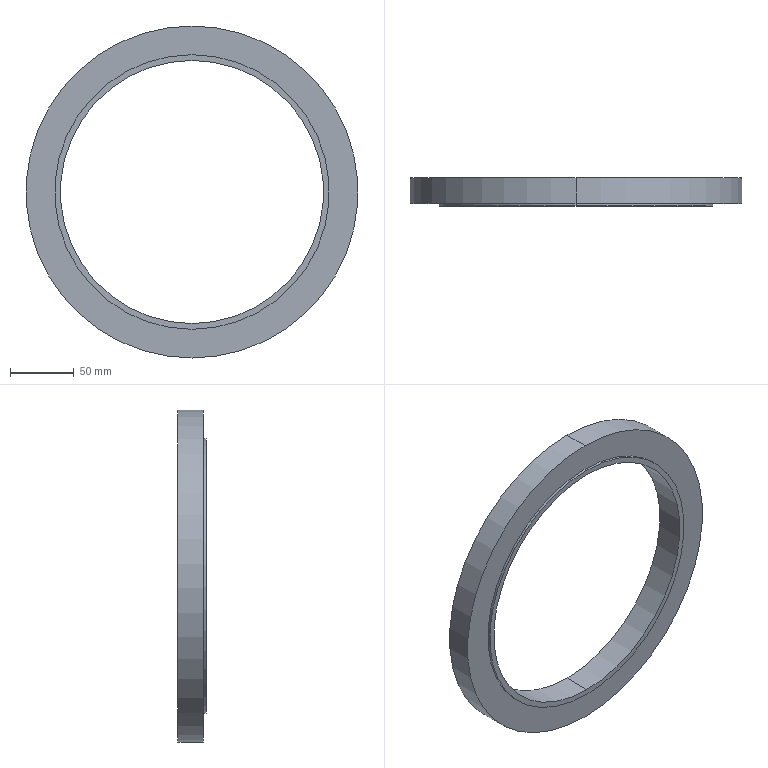Part | SolidWorks | features CirPattern 1, FlatPattern 1, HoleWzd 1, ICE 1, SMBaseFlange 1, SheetMetal 1 | 1 solid | 33 faces | box 260 x 22 x 260 mm | volume 392882 mm3 | cylinder 18 | cone 12 | plane 3 | commonest cylinder face diameters 10.2 x12 206 x2 215 x2 260 x2
STEP:
#1=CARTESIAN_POINT('',(99.593,-16.,-62.6));
#2=VERTEX_POINT('',#1);
#3=CARTESIAN_POINT('',(99.593,-16.,-52.4));
#4=VERTEX_POINT('',#3);
#5=CARTESIAN_POINT('',(99.593,-16.,-57.5));
#6=DIRECTION('',(0.,1.,0.));
#7=DIRECTION('',(0.,0.,1.));
#8=AXIS2_PLACEMENT_3D('',#5,#6,#7);
#9=CIRCLE('',#8,5.1);
#10=EDGE_CURVE('',#2,#4,#9,.T.);
#11=ORIENTED_EDGE('',*,*,#10,.F.);
#12=CARTESIAN_POINT('',(99.593,0.,-62.6));
#13=VERTEX_POINT('',#12);
#14=CARTESIAN_POINT('',(99.593,0.,-62.6));
#15=DIRECTION('',(0.,1.,0.));
#16=VECTOR('',#15,1000.);
#17=LINE('',#14,#16);
#18=EDGE_CURVE('',#2,#13,#17,.T.);
#19=ORIENTED_EDGE('',*,*,#18,.T.);
#20=CARTESIAN_POINT('',(99.593,0.,-52.4));
#21=VERTEX_POINT('',#20);
#22=CARTESIAN_POINT('',(99.593,0.,-57.5));
#23=DIRECTION('',(0.,1.,0.));
#24=DIRECTION('',(0.,0.,1.));
#25=AXIS2_PLACEMENT_3D('',#22,#23,#24);
#26=CIRCLE('',#25,5.1);
#27=EDGE_CURVE('',#13,#21,#26,.T.);
#28=ORIENTED_EDGE('',*,*,#27,.T.);
#29=CARTESIAN_POINT('',(99.593,0.,-52.4));
#30=DIRECTION('',(0.,1.,0.));
#31=VECTOR('',#30,1000.);
#32=LINE('',#29,#31);
#33=EDGE_CURVE('',#4,#21,#32,.T.);
#34=ORIENTED_EDGE('',*,*,#33,.F.);
#35=EDGE_LOOP('',(#11,#19,#28,#34));
#36=FACE_OUTER_BOUND('',#35,.T.);
#37=CARTESIAN_POINT('',(99.593,0.,-57.5));
#38=DIRECTION('',(0.,1.,0.));
#39=DIRECTION('',(0.,0.,1.));
#40=AXIS2_PLACEMENT_3D('',#37,#38,#39);
#41=CYLINDRICAL_SURFACE('',#40,5.1);
#42=ADVANCED_FACE('',(#36),#41,.F.);
#43=CARTESIAN_POINT('',(99.593,-19.064,-57.5));
#44=VERTEX_POINT('',#43);
#45=CARTESIAN_POINT('',(99.593,-16.,-52.4));
#46=DIRECTION('',(0.,0.515,0.8572));
#47=VECTOR('',#46,1000.);
#48=LINE('',#45,#47);
#49=EDGE_CURVE('',#44,#4,#48,.T.);
#50=ORIENTED_EDGE('',*,*,#49,.F.);
#51=CARTESIAN_POINT('',(99.593,-16.,-62.6));
#52=DIRECTION('',(0.,0.515,-0.8572));
#53=VECTOR('',#52,1000.);
#54=LINE('',#51,#53);
#55=EDGE_CURVE('',#44,#2,#54,.T.);
#56=ORIENTED_EDGE('',*,*,#55,.T.);
#57=ORIENTED_EDGE('',*,*,#10,.T.);
#58=EDGE_LOOP('',(#50,#56,#57));
#59=FACE_OUTER_BOUND('',#58,.T.);
#60=CARTESIAN_POINT('',(99.593,-16.,-57.5));
#61=DIRECTION('',(0.,1.,0.));
#62=DIRECTION('',(0.,0.,1.));
#63=AXIS2_PLACEMENT_3D('',#60,#61,#62);
#64=CONICAL_SURFACE('',#63,5.1,1.03);
#65=ADVANCED_FACE('',(#59),#64,.F.);
#66=CARTESIAN_POINT('',(99.593,-16.,52.4));
#67=VERTEX_POINT('',#66);
#68=CARTESIAN_POINT('',(99.593,-16.,62.6));
#69=VERTEX_POINT('',#68);
#70=CARTESIAN_POINT('',(99.593,-16.,57.5));
#71=DIRECTION('',(0.,1.,0.));
#72=DIRECTION('',(0.,0.,1.));
#73=AXIS2_PLACEMENT_3D('',#70,#71,#72);
#74=CIRCLE('',#73,5.1);
#75=EDGE_CURVE('',#67,#69,#74,.T.);
#76=ORIENTED_EDGE('',*,*,#75,.F.);
#77=CARTESIAN_POINT('',(99.593,0.,52.4));
#78=VERTEX_POINT('',#77);
#79=CARTESIAN_POINT('',(99.593,0.,52.4));
#80=DIRECTION('',(0.,1.,0.));
#81=VECTOR('',#80,1000.);
#82=LINE('',#79,#81);
#83=EDGE_CURVE('',#67,#78,#82,.T.);
#84=ORIENTED_EDGE('',*,*,#83,.T.);
#85=CARTESIAN_POINT('',(99.593,0.,62.6));
#86=VERTEX_POINT('',#85);
#87=CARTESIAN_POINT('',(99.593,0.,57.5));
#88=DIRECTION('',(0.,1.,0.));
#89=DIRECTION('',(0.,0.,1.));
#90=AXIS2_PLACEMENT_3D('',#87,#88,#89);
#91=CIRCLE('',#90,5.1);
#92=EDGE_CURVE('',#78,#86,#91,.T.);
#93=ORIENTED_EDGE('',*,*,#92,.T.);
#94=CARTESIAN_POINT('',(99.593,0.,62.6));
#95=DIRECTION('',(0.,1.,0.));
#96=VECTOR('',#95,1000.);
#97=LINE('',#94,#96);
#98=EDGE_CURVE('',#69,#86,#97,.T.);
#99=ORIENTED_EDGE('',*,*,#98,.F.);
#100=EDGE_LOOP('',(#76,#84,#93,#99));
#101=FACE_OUTER_BOUND('',#100,.T.);
#102=CARTESIAN_POINT('',(99.593,0.,57.5));
#103=DIRECTION('',(0.,1.,0.));
#104=DIRECTION('',(0.,0.,1.));
#105=AXIS2_PLACEMENT_3D('',#102,#103,#104);
#106=CYLINDRICAL_SURFACE('',#105,5.1);
#107=ADVANCED_FACE('',(#101),#106,.F.);
#108=CARTESIAN_POINT('',(99.593,-19.064,57.5));
#109=VERTEX_POINT('',#108);
#110=CARTESIAN_POINT('',(99.593,-16.,62.6));
#111=DIRECTION('',(0.,0.515,0.8572));
#112=VECTOR('',#111,1000.);
#113=LINE('',#110,#112);
#114=EDGE_CURVE('',#109,#69,#113,.T.);
#115=ORIENTED_EDGE('',*,*,#114,.F.);
#116=CARTESIAN_POINT('',(99.593,-16.,52.4));
#117=DIRECTION('',(0.,0.515,-0.8572));
#118=VECTOR('',#117,1000.);
#119=LINE('',#116,#118);
#120=EDGE_CURVE('',#109,#67,#119,.T.);
#121=ORIENTED_EDGE('',*,*,#120,.T.);
#122=ORIENTED_EDGE('',*,*,#75,.T.);
#123=EDGE_LOOP('',(#115,#121,#122));
#124=FACE_OUTER_BOUND('',#123,.T.);
#125=CARTESIAN_POINT('',(99.593,-16.,57.5));
#126=DIRECTION('',(0.,1.,0.));
#127=DIRECTION('',(0.,0.,1.));
#128=AXIS2_PLACEMENT_3D('',#125,#126,#127);
#129=CONICAL_SURFACE('',#128,5.1,1.03);
#130=ADVANCED_FACE('',(#124),#129,.F.);
#131=CARTESIAN_POINT('',(0.,-16.,109.9));
#132=VERTEX_POINT('',#131);
#133=CARTESIAN_POINT('',(0.,-16.,120.1));
#134=VERTEX_POINT('',#133);
#135=CARTESIAN_POINT('',(0.,-16.,115.));
#136=DIRECTION('',(0.,1.,0.));
#137=DIRECTION('',(0.,0.,1.));
#138=AXIS2_PLACEMENT_3D('',#135,#136,#137);
#139=CIRCLE('',#138,5.1);
#140=EDGE_CURVE('',#132,#134,#139,.T.);
#141=ORIENTED_EDGE('',*,*,#140,.F.);
#142=CARTESIAN_POINT('',(0.,0.,109.9));
#143=VERTEX_POINT('',#142);
#144=CARTESIAN_POINT('',(0.,0.,109.9));
#145=DIRECTION('',(0.,1.,0.));
#146=VECTOR('',#145,1000.);
#147=LINE('',#144,#146);
#148=EDGE_CURVE('',#132,#143,#147,.T.);
#149=ORIENTED_EDGE('',*,*,#148,.T.);
#150=CARTESIAN_POINT('',(0.,0.,120.1));
#151=VERTEX_POINT('',#150);
#152=CARTESIAN_POINT('',(0.,0.,115.));
#153=DIRECTION('',(0.,1.,0.));
#154=DIRECTION('',(0.,0.,1.));
#155=AXIS2_PLACEMENT_3D('',#152,#153,#154);
#156=CIRCLE('',#155,5.1);
#157=EDGE_CURVE('',#143,#151,#156,.T.);
#158=ORIENTED_EDGE('',*,*,#157,.T.);
#159=CARTESIAN_POINT('',(0.,0.,120.1));
#160=DIRECTION('',(0.,1.,0.));
#161=VECTOR('',#160,1000.);
#162=LINE('',#159,#161);
#163=EDGE_CURVE('',#134,#151,#162,.T.);
#164=ORIENTED_EDGE('',*,*,#163,.F.);
#165=EDGE_LOOP('',(#141,#149,#158,#164));
#166=FACE_OUTER_BOUND('',#165,.T.);
#167=CARTESIAN_POINT('',(0.,0.,115.));
#168=DIRECTION('',(0.,1.,0.));
#169=DIRECTION('',(0.,0.,1.));
#170=AXIS2_PLACEMENT_3D('',#167,#168,#169);
#171=CYLINDRICAL_SURFACE('',#170,5.1);
#172=ADVANCED_FACE('',(#166),#171,.F.);
#173=CARTESIAN_POINT('',(0.,-19.064,115.));
#174=VERTEX_POINT('',#173);
#175=CARTESIAN_POINT('',(0.,-16.,120.1));
#176=DIRECTION('',(0.,0.515,0.8572));
#177=VECTOR('',#176,1000.);
#178=LINE('',#175,#177);
#179=EDGE_CURVE('',#174,#134,#178,.T.);
#180=ORIENTED_EDGE('',*,*,#179,.F.);
#181=CARTESIAN_POINT('',(0.,-16.,109.9));
#182=DIRECTION('',(0.,0.515,-0.8572));
#183=VECTOR('',#182,1000.);
#184=LINE('',#181,#183);
#185=EDGE_CURVE('',#174,#132,#184,.T.);
#186=ORIENTED_EDGE('',*,*,#185,.T.);
#187=ORIENTED_EDGE('',*,*,#140,.T.);
#188=EDGE_LOOP('',(#180,#186,#187));
#189=FACE_OUTER_BOUND('',#188,.T.);
#190=CARTESIAN_POINT('',(0.,-16.,115.));
#191=DIRECTION('',(0.,1.,0.));
#192=DIRECTION('',(0.,0.,1.));
#193=AXIS2_PLACEMENT_3D('',#190,#191,#192);
#194=CONICAL_SURFACE('',#193,5.1,1.03);
#195=ADVANCED_FACE('',(#189),#194,.F.);
#196=CARTESIAN_POINT('',(-99.593,-16.,52.4));
#197=VERTEX_POINT('',#196);
#198=CARTESIAN_POINT('',(-99.593,-16.,62.6));
#199=VERTEX_POINT('',#198);
#200=CARTESIAN_POINT('',(-99.593,-16.,57.5));
#201=DIRECTION('',(0.,1.,0.));
#202=DIRECTION('',(0.,0.,1.));
#203=AXIS2_PLACEMENT_3D('',#200,#201,#202);
#204=CIRCLE('',#203,5.1);
#205=EDGE_CURVE('',#197,#199,#204,.T.);
#206=ORIENTED_EDGE('',*,*,#205,.F.);
#207=CARTESIAN_POINT('',(-99.593,0.,52.4));
#208=VERTEX_POINT('',#207);
#209=CARTESIAN_POINT('',(-99.593,0.,52.4));
#210=DIRECTION('',(0.,1.,0.));
#211=VECTOR('',#210,1000.);
#212=LINE('',#209,#211);
#213=EDGE_CURVE('',#197,#208,#212,.T.);
#214=ORIENTED_EDGE('',*,*,#213,.T.);
#215=CARTESIAN_POINT('',(-99.593,0.,62.6));
#216=VERTEX_POINT('',#215);
#217=CARTESIAN_POINT('',(-99.593,0.,57.5));
#218=DIRECTION('',(0.,1.,0.));
#219=DIRECTION('',(0.,0.,1.));
#220=AXIS2_PLACEMENT_3D('',#217,#218,#219);
#221=CIRCLE('',#220,5.1);
#222=EDGE_CURVE('',#208,#216,#221,.T.);
#223=ORIENTED_EDGE('',*,*,#222,.T.);
#224=CARTESIAN_POINT('',(-99.593,0.,62.6));
#225=DIRECTION('',(0.,1.,0.));
#226=VECTOR('',#225,1000.);
#227=LINE('',#224,#226);
#228=EDGE_CURVE('',#199,#216,#227,.T.);
#229=ORIENTED_EDGE('',*,*,#228,.F.);
#230=EDGE_LOOP('',(#206,#214,#223,#229));
#231=FACE_OUTER_BOUND('',#230,.T.);
#232=CARTESIAN_POINT('',(-99.593,0.,57.5));
#233=DIRECTION('',(0.,1.,0.));
#234=DIRECTION('',(0.,0.,1.));
#235=AXIS2_PLACEMENT_3D('',#232,#233,#234);
#236=CYLINDRICAL_SURFACE('',#235,5.1);
#237=ADVANCED_FACE('',(#231),#236,.F.);
#238=CARTESIAN_POINT('',(-99.593,-19.064,57.5));
#239=VERTEX_POINT('',#238);
#240=CARTESIAN_POINT('',(-99.593,-16.,62.6));
#241=DIRECTION('',(0.,0.515,0.8572));
#242=VECTOR('',#241,1000.);
#243=LINE('',#240,#242);
#244=EDGE_CURVE('',#239,#199,#243,.T.);
#245=ORIENTED_EDGE('',*,*,#244,.F.);
#246=CARTESIAN_POINT('',(-99.593,-16.,52.4));
#247=DIRECTION('',(0.,0.515,-0.8572));
#248=VECTOR('',#247,1000.);
#249=LINE('',#246,#248);
#250=EDGE_CURVE('',#239,#197,#249,.T.);
#251=ORIENTED_EDGE('',*,*,#250,.T.);
#252=ORIENTED_EDGE('',*,*,#205,.T.);
#253=EDGE_LOOP('',(#245,#251,#252));
#254=FACE_OUTER_BOUND('',#253,.T.);
#255=CARTESIAN_POINT('',(-99.593,-16.,57.5));
#256=DIRECTION('',(0.,1.,0.));
#257=DIRECTION('',(0.,0.,1.));
#258=AXIS2_PLACEMENT_3D('',#255,#256,#257);
#259=CONICAL_SURFACE('',#258,5.1,1.03);
#260=ADVANCED_FACE('',(#254),#259,.F.);
#261=CARTESIAN_POINT('',(-99.593,-16.,-62.6));
#262=VERTEX_POINT('',#261);
#263=CARTESIAN_POINT('',(-99.593,-16.,-52.4));
#264=VERTEX_POINT('',#263);
#265=CARTESIAN_POINT('',(-99.593,-16.,-57.5));
#266=DIRECTION('',(0.,1.,0.));
#267=DIRECTION('',(0.,0.,1.));
#268=AXIS2_PLACEMENT_3D('',#265,#266,#267);
#269=CIRCLE('',#268,5.1);
#270=EDGE_CURVE('',#262,#264,#269,.T.);
#271=ORIENTED_EDGE('',*,*,#270,.F.);
#272=CARTESIAN_POINT('',(-99.593,0.,-62.6));
#273=VERTEX_POINT('',#272);
#274=CARTESIAN_POINT('',(-99.593,0.,-62.6));
#275=DIRECTION('',(0.,1.,0.));
#276=VECTOR('',#275,1000.);
#277=LINE('',#274,#276);
#278=EDGE_CURVE('',#262,#273,#277,.T.);
#279=ORIENTED_EDGE('',*,*,#278,.T.);
#280=CARTESIAN_POINT('',(-99.593,0.,-52.4));
#281=VERTEX_POINT('',#280);
#282=CARTESIAN_POINT('',(-99.593,0.,-57.5));
#283=DIRECTION('',(0.,1.,0.));
#284=DIRECTION('',(0.,0.,1.));
#285=AXIS2_PLACEMENT_3D('',#282,#283,#284);
#286=CIRCLE('',#285,5.1);
#287=EDGE_CURVE('',#273,#281,#286,.T.);
#288=ORIENTED_EDGE('',*,*,#287,.T.);
#289=CARTESIAN_POINT('',(-99.593,0.,-52.4));
#290=DIRECTION('',(0.,1.,0.));
#291=VECTOR('',#290,1000.);
#292=LINE('',#289,#291);
#293=EDGE_CURVE('',#264,#281,#292,.T.);
#294=ORIENTED_EDGE('',*,*,#293,.F.);
#295=EDGE_LOOP('',(#271,#279,#288,#294));
#296=FACE_OUTER_BOUND('',#295,.T.);
#297=CARTESIAN_POINT('',(-99.593,0.,-57.5));
#298=DIRECTION('',(0.,1.,0.));
#299=DIRECTION('',(0.,0.,1.));
#300=AXIS2_PLACEMENT_3D('',#297,#298,#299);
#301=CYLINDRICAL_SURFACE('',#300,5.1);
#302=ADVANCED_FACE('',(#296),#301,.F.);
#303=CARTESIAN_POINT('',(-99.593,-19.064,-57.5));
#304=VERTEX_POINT('',#303);
#305=CARTESIAN_POINT('',(-99.593,-16.,-52.4));
#306=DIRECTION('',(0.,0.515,0.8572));
#307=VECTOR('',#306,1000.);
#308=LINE('',#305,#307);
#309=EDGE_CURVE('',#304,#264,#308,.T.);
#310=ORIENTED_EDGE('',*,*,#309,.F.);
#311=CARTESIAN_POINT('',(-99.593,-16.,-62.6));
#312=DIRECTION('',(0.,0.515,-0.8572));
#313=VECTOR('',#312,1000.);
#314=LINE('',#311,#313);
#315=EDGE_CURVE('',#304,#262,#314,.T.);
#316=ORIENTED_EDGE('',*,*,#315,.T.);
#317=ORIENTED_EDGE('',*,*,#270,.T.);
#318=EDGE_LOOP('',(#310,#316,#317));
#319=FACE_OUTER_BOUND('',#318,.T.);
#320=CARTESIAN_POINT('',(-99.593,-16.,-57.5));
#321=DIRECTION('',(0.,1.,0.));
#322=DIRECTION('',(0.,0.,1.));
#323=AXIS2_PLACEMENT_3D('',#320,#321,#322);
#324=CONICAL_SURFACE('',#323,5.1,1.03);
#325=ADVANCED_FACE('',(#319),#324,.F.);
#326=CARTESIAN_POINT('',(0.,-16.,-120.1));
#327=VERTEX_POINT('',#326);
#328=CARTESIAN_POINT('',(0.,-16.,-109.9));
#329=VERTEX_POINT('',#328);
#330=CARTESIAN_POINT('',(0.,-16.,-115.));
#331=DIRECTION('',(0.,1.,0.));
#332=DIRECTION('',(0.,0.,1.));
#333=AXIS2_PLACEMENT_3D('',#330,#331,#332);
#334=CIRCLE('',#333,5.1);
#335=EDGE_CURVE('',#327,#329,#334,.T.);
#336=ORIENTED_EDGE('',*,*,#335,.F.);
#337=CARTESIAN_POINT('',(0.,0.,-120.1));
#338=VERTEX_POINT('',#337);
#339=CARTESIAN_POINT('',(0.,0.,-120.1));
#340=DIRECTION('',(0.,1.,0.));
#341=VECTOR('',#340,1000.);
#342=LINE('',#339,#341);
#343=EDGE_CURVE('',#327,#338,#342,.T.);
#344=ORIENTED_EDGE('',*,*,#343,.T.);
#345=CARTESIAN_POINT('',(0.,0.,-109.9));
#346=VERTEX_POINT('',#345);
#347=CARTESIAN_POINT('',(0.,0.,-115.));
#348=DIRECTION('',(0.,1.,0.));
#349=DIRECTION('',(0.,0.,1.));
#350=AXIS2_PLACEMENT_3D('',#347,#348,#349);
#351=CIRCLE('',#350,5.1);
#352=EDGE_CURVE('',#338,#346,#351,.T.);
#353=ORIENTED_EDGE('',*,*,#352,.T.);
#354=CARTESIAN_POINT('',(0.,0.,-109.9));
#355=DIRECTION('',(0.,1.,0.));
#356=VECTOR('',#355,1000.);
#357=LINE('',#354,#356);
#358=EDGE_CURVE('',#329,#346,#357,.T.);
#359=ORIENTED_EDGE('',*,*,#358,.F.);
#360=EDGE_LOOP('',(#336,#344,#353,#359));
#361=FACE_OUTER_BOUND('',#360,.T.);
#362=CARTESIAN_POINT('',(0.,0.,-115.));
#363=DIRECTION('',(0.,1.,0.));
#364=DIRECTION('',(0.,0.,1.));
#365=AXIS2_PLACEMENT_3D('',#362,#363,#364);
#366=CYLINDRICAL_SURFACE('',#365,5.1);
#367=ADVANCED_FACE('',(#361),#366,.F.);
#368=CARTESIAN_POINT('',(0.,-19.064,-115.));
#369=VERTEX_POINT('',#368);
#370=CARTESIAN_POINT('',(0.,-16.,-109.9));
#371=DIRECTION('',(0.,0.515,0.8572));
#372=VECTOR('',#371,1000.);
#373=LINE('',#370,#372);
#374=EDGE_CURVE('',#369,#329,#373,.T.);
#375=ORIENTED_EDGE('',*,*,#374,.F.);
#376=CARTESIAN_POINT('',(0.,-16.,-120.1));
#377=DIRECTION('',(0.,0.515,-0.8572));
#378=VECTOR('',#377,1000.);
#379=LINE('',#376,#378);
#380=EDGE_CURVE('',#369,#327,#379,.T.);
#381=ORIENTED_EDGE('',*,*,#380,.T.);
#382=ORIENTED_EDGE('',*,*,#335,.T.);
#383=EDGE_LOOP('',(#375,#381,#382));
#384=FACE_OUTER_BOUND('',#383,.T.);
#385=CARTESIAN_POINT('',(0.,-16.,-115.));
#386=DIRECTION('',(0.,1.,0.));
#387=DIRECTION('',(0.,0.,1.));
#388=AXIS2_PLACEMENT_3D('',#385,#386,#387);
#389=CONICAL_SURFACE('',#388,5.1,1.03);
#390=ADVANCED_FACE('',(#384),#389,.F.);
#391=CARTESIAN_POINT('',(0.,-20.,-107.5));
#392=VERTEX_POINT('',#391);
#393=CARTESIAN_POINT('',(0.,-20.,107.5));
#394=VERTEX_POINT('',#393);
#395=CARTESIAN_POINT('',(0.,-20.,0.));
#396=DIRECTION('',(0.,-1.,0.));
#397=DIRECTION('',(0.,0.,-1.));
#398=AXIS2_PLACEMENT_3D('',#395,#396,#397);
#399=CIRCLE('',#398,107.5);
#400=EDGE_CURVE('',#392,#394,#399,.T.);
#401=ORIENTED_EDGE('',*,*,#400,.T.);
#402=CARTESIAN_POINT('',(0.,-22.,107.5));
#403=VERTEX_POINT('',#402);
#404=CARTESIAN_POINT('',(0.,-20.,107.5));
#405=DIRECTION('',(0.,-1.,0.));
#406=VECTOR('',#405,1000.);
#407=LINE('',#404,#406);
#408=EDGE_CURVE('',#394,#403,#407,.T.);
#409=ORIENTED_EDGE('',*,*,#408,.T.);
#410=CARTESIAN_POINT('',(0.,-22.,-107.5));
#411=VERTEX_POINT('',#410);
#412=CARTESIAN_POINT('',(0.,-22.,0.));
#413=DIRECTION('',(0.,-1.,0.));
#414=DIRECTION('',(0.,0.,-1.));
#415=AXIS2_PLACEMENT_3D('',#412,#413,#414);
#416=CIRCLE('',#415,107.5);
#417=EDGE_CURVE('',#411,#403,#416,.T.);
#418=ORIENTED_EDGE('',*,*,#417,.F.);
#419=CARTESIAN_POINT('',(0.,-20.,-107.5));
#420=DIRECTION('',(0.,-1.,0.));
#421=VECTOR('',#420,1000.);
#422=LINE('',#419,#421);
#423=EDGE_CURVE('',#392,#411,#422,.T.);
#424=ORIENTED_EDGE('',*,*,#423,.F.);
#425=EDGE_LOOP('',(#401,#409,#418,#424));
#426=FACE_OUTER_BOUND('',#425,.T.);
#427=CARTESIAN_POINT('',(0.,-20.,0.));
#428=DIRECTION('',(0.,-1.,0.));
#429=DIRECTION('',(0.,0.,-1.));
#430=AXIS2_PLACEMENT_3D('',#427,#428,#429);
#431=CYLINDRICAL_SURFACE('',#430,107.5);
#432=ADVANCED_FACE('',(#426),#431,.T.);
#433=CARTESIAN_POINT('',(0.,-22.,-103.));
#434=VERTEX_POINT('',#433);
#435=CARTESIAN_POINT('',(0.,-22.,103.));
#436=VERTEX_POINT('',#435);
#437=CARTESIAN_POINT('',(0.,-22.,0.));
#438=DIRECTION('',(0.,1.,0.));
#439=DIRECTION('',(0.,0.,1.));
#440=AXIS2_PLACEMENT_3D('',#437,#438,#439);
#441=CIRCLE('',#440,103.);
#442=EDGE_CURVE('',#434,#436,#441,.T.);
#443=ORIENTED_EDGE('',*,*,#442,.F.);
#444=CARTESIAN_POINT('',(0.,0.,-103.));
#445=VERTEX_POINT('',#444);
#446=CARTESIAN_POINT('',(0.,-22.,-103.));
#447=DIRECTION('',(0.,1.,0.));
#448=VECTOR('',#447,1000.);
#449=LINE('',#446,#448);
#450=EDGE_CURVE('',#434,#445,#449,.T.);
#451=ORIENTED_EDGE('',*,*,#450,.T.);
#452=CARTESIAN_POINT('',(0.,0.,103.));
#453=VERTEX_POINT('',#452);
#454=CARTESIAN_POINT('',(0.,0.,0.));
#455=DIRECTION('',(0.,1.,0.));
#456=DIRECTION('',(0.,0.,1.));
#457=AXIS2_PLACEMENT_3D('',#454,#455,#456);
#458=CIRCLE('',#457,103.);
#459=EDGE_CURVE('',#445,#453,#458,.T.);
#460=ORIENTED_EDGE('',*,*,#459,.T.);
#461=CARTESIAN_POINT('',(0.,-22.,103.));
#462=DIRECTION('',(0.,1.,0.));
#463=VECTOR('',#462,1000.);
#464=LINE('',#461,#463);
#465=EDGE_CURVE('',#436,#453,#464,.T.);
#466=ORIENTED_EDGE('',*,*,#465,.F.);
#467=EDGE_LOOP('',(#443,#451,#460,#466));
#468=FACE_OUTER_BOUND('',#467,.T.);
#469=CARTESIAN_POINT('',(0.,-22.,0.));
#470=DIRECTION('',(0.,1.,0.));
#471=DIRECTION('',(0.,0.,1.));
#472=AXIS2_PLACEMENT_3D('',#469,#470,#471);
#473=CYLINDRICAL_SURFACE('',#472,103.);
#474=ADVANCED_FACE('',(#468),#473,.F.);
#475=CARTESIAN_POINT('',(0.,-20.,130.));
#476=VERTEX_POINT('',#475);
#477=CARTESIAN_POINT('',(0.,-20.,-130.));
#478=VERTEX_POINT('',#477);
#479=CARTESIAN_POINT('',(0.,-20.,0.));
#480=DIRECTION('',(0.,1.,0.));
#481=DIRECTION('',(0.,0.,-1.));
#482=AXIS2_PLACEMENT_3D('',#479,#480,#481);
#483=CIRCLE('',#482,130.);
#484=EDGE_CURVE('',#476,#478,#483,.T.);
#485=ORIENTED_EDGE('',*,*,#484,.T.);
#486=CARTESIAN_POINT('',(0.,0.,-130.));
#487=VERTEX_POINT('',#486);
#488=CARTESIAN_POINT('',(0.,-22.,-130.));
#489=DIRECTION('',(0.,1.,0.));
#490=VECTOR('',#489,1000.);
#491=LINE('',#488,#490);
#492=EDGE_CURVE('',#478,#487,#491,.T.);
#493=ORIENTED_EDGE('',*,*,#492,.T.);
#494=CARTESIAN_POINT('',(0.,0.,130.));
#495=VERTEX_POINT('',#494);
#496=CARTESIAN_POINT('',(0.,0.,0.));
#497=DIRECTION('',(0.,1.,0.));
#498=DIRECTION('',(0.,0.,1.));
#499=AXIS2_PLACEMENT_3D('',#496,#497,#498);
#500=CIRCLE('',#499,130.);
#501=EDGE_CURVE('',#495,#487,#500,.T.);
#502=ORIENTED_EDGE('',*,*,#501,.F.);
#503=CARTESIAN_POINT('',(0.,-22.,130.));
#504=DIRECTION('',(0.,1.,0.));
#505=VECTOR('',#504,1000.);
#506=LINE('',#503,#505);
#507=EDGE_CURVE('',#476,#495,#506,.T.);
#508=ORIENTED_EDGE('',*,*,#507,.F.);
#509=EDGE_LOOP('',(#485,#493,#502,#508));
#510=FACE_OUTER_BOUND('',#509,.T.);
#511=CARTESIAN_POINT('',(0.,-22.,0.));
#512=DIRECTION('',(0.,1.,0.));
#513=DIRECTION('',(0.,0.,1.));
#514=AXIS2_PLACEMENT_3D('',#511,#512,#513);
#515=CYLINDRICAL_SURFACE('',#514,130.);
#516=ADVANCED_FACE('',(#510),#515,.T.);
#517=ORIENTED_EDGE('',*,*,#492,.F.);
#518=CARTESIAN_POINT('',(0.,-20.,0.));
#519=DIRECTION('',(0.,1.,0.));
#520=DIRECTION('',(0.,0.,-1.));
#521=AXIS2_PLACEMENT_3D('',#518,#519,#520);
#522=CIRCLE('',#521,130.);
#523=EDGE_CURVE('',#478,#476,#522,.T.);
#524=ORIENTED_EDGE('',*,*,#523,.T.);
#525=ORIENTED_EDGE('',*,*,#507,.T.);
#526=CARTESIAN_POINT('',(0.,0.,0.));
#527=DIRECTION('',(0.,1.,0.));
#528=DIRECTION('',(0.,0.,1.));
#529=AXIS2_PLACEMENT_3D('',#526,#527,#528);
#530=CIRCLE('',#529,130.);
#531=EDGE_CURVE('',#487,#495,#530,.T.);
#532=ORIENTED_EDGE('',*,*,#531,.F.);
#533=EDGE_LOOP('',(#517,#524,#525,#532));
#534=FACE_OUTER_BOUND('',#533,.T.);
#535=CARTESIAN_POINT('',(0.,-22.,0.));
#536=DIRECTION('',(0.,1.,0.));
#537=DIRECTION('',(0.,0.,1.));
#538=AXIS2_PLACEMENT_3D('',#535,#536,#537);
#539=CYLINDRICAL_SURFACE('',#538,130.);
#540=ADVANCED_FACE('',(#534),#539,.T.);
#541=CARTESIAN_POINT('',(0.,-22.,0.));
#542=DIRECTION('',(0.,1.,0.));
#543=DIRECTION('',(0.,0.,1.));
#544=AXIS2_PLACEMENT_3D('',#541,#542,#543);
#545=CIRCLE('',#544,103.);
#546=EDGE_CURVE('',#436,#434,#545,.T.);
#547=ORIENTED_EDGE('',*,*,#546,.T.);
#548=ORIENTED_EDGE('',*,*,#442,.T.);
#549=EDGE_LOOP('',(#547,#548));
#550=FACE_BOUND('',#549,.T.);
#551=ORIENTED_EDGE('',*,*,#417,.T.);
#552=CARTESIAN_POINT('',(0.,-22.,0.));
#553=DIRECTION('',(0.,-1.,0.));
#554=DIRECTION('',(0.,0.,-1.));
#555=AXIS2_PLACEMENT_3D('',#552,#553,#554);
#556=CIRCLE('',#555,107.5);
#557=EDGE_CURVE('',#403,#411,#556,.T.);
#558=ORIENTED_EDGE('',*,*,#557,.T.);
#559=EDGE_LOOP('',(#551,#558));
#560=FACE_OUTER_BOUND('',#559,.T.);
#561=CARTESIAN_POINT('',(0.,-22.,0.));
#562=DIRECTION('',(0.,1.,0.));
#563=DIRECTION('',(0.,0.,1.));
#564=AXIS2_PLACEMENT_3D('',#561,#562,#563);
#565=PLANE('',#564);
#566=ADVANCED_FACE('',(#550,#560),#565,.F.);
#567=CARTESIAN_POINT('',(99.593,0.,-57.5));
#568=DIRECTION('',(0.,1.,0.));
#569=DIRECTION('',(0.,0.,1.));
#570=AXIS2_PLACEMENT_3D('',#567,#568,#569);
#571=CIRCLE('',#570,5.1);
#572=EDGE_CURVE('',#21,#13,#571,.T.);
#573=ORIENTED_EDGE('',*,*,#572,.F.);
#574=ORIENTED_EDGE('',*,*,#27,.F.);
#575=EDGE_LOOP('',(#573,#574));
#576=FACE_BOUND('',#575,.T.);
#577=CARTESIAN_POINT('',(99.593,0.,57.5));
#578=DIRECTION('',(0.,1.,0.));
#579=DIRECTION('',(0.,0.,1.));
#580=AXIS2_PLACEMENT_3D('',#577,#578,#579);
#581=CIRCLE('',#580,5.1);
#582=EDGE_CURVE('',#86,#78,#581,.T.);
#583=ORIENTED_EDGE('',*,*,#582,.F.);
#584=ORIENTED_EDGE('',*,*,#92,.F.);
#585=EDGE_LOOP('',(#583,#584));
#586=FACE_BOUND('',#585,.T.);
#587=CARTESIAN_POINT('',(0.,0.,115.));
#588=DIRECTION('',(0.,1.,0.));
#589=DIRECTION('',(0.,0.,1.));
#590=AXIS2_PLACEMENT_3D('',#587,#588,#589);
#591=CIRCLE('',#590,5.1);
#592=EDGE_CURVE('',#151,#143,#591,.T.);
#593=ORIENTED_EDGE('',*,*,#592,.F.);
#594=ORIENTED_EDGE('',*,*,#157,.F.);
#595=EDGE_LOOP('',(#593,#594));
#596=FACE_BOUND('',#595,.T.);
#597=CARTESIAN_POINT('',(-99.593,0.,57.5));
#598=DIRECTION('',(0.,1.,0.));
#599=DIRECTION('',(0.,0.,1.));
#600=AXIS2_PLACEMENT_3D('',#597,#598,#599);
#601=CIRCLE('',#600,5.1);
#602=EDGE_CURVE('',#216,#208,#601,.T.);
#603=ORIENTED_EDGE('',*,*,#602,.F.);
#604=ORIENTED_EDGE('',*,*,#222,.F.);
#605=EDGE_LOOP('',(#603,#604));
#606=FACE_BOUND('',#605,.T.);
#607=CARTESIAN_POINT('',(-99.593,0.,-57.5));
#608=DIRECTION('',(0.,1.,0.));
#609=DIRECTION('',(0.,0.,1.));
#610=AXIS2_PLACEMENT_3D('',#607,#608,#609);
#611=CIRCLE('',#610,5.1);
#612=EDGE_CURVE('',#281,#273,#611,.T.);
#613=ORIENTED_EDGE('',*,*,#612,.F.);
#614=ORIENTED_EDGE('',*,*,#287,.F.);
#615=EDGE_LOOP('',(#613,#614));
#616=FACE_BOUND('',#615,.T.);
#617=CARTESIAN_POINT('',(0.,0.,-115.));
#618=DIRECTION('',(0.,1.,0.));
#619=DIRECTION('',(0.,0.,1.));
#620=AXIS2_PLACEMENT_3D('',#617,#618,#619);
#621=CIRCLE('',#620,5.1);
#622=EDGE_CURVE('',#346,#338,#621,.T.);
#623=ORIENTED_EDGE('',*,*,#622,.F.);
#624=ORIENTED_EDGE('',*,*,#352,.F.);
#625=EDGE_LOOP('',(#623,#624));
#626=FACE_BOUND('',#625,.T.);
#627=CARTESIAN_POINT('',(0.,0.,0.));
#628=DIRECTION('',(0.,1.,0.));
#629=DIRECTION('',(0.,0.,1.));
#630=AXIS2_PLACEMENT_3D('',#627,#628,#629);
#631=CIRCLE('',#630,103.);
#632=EDGE_CURVE('',#453,#445,#631,.T.);
#633=ORIENTED_EDGE('',*,*,#632,.F.);
#634=ORIENTED_EDGE('',*,*,#459,.F.);
#635=EDGE_LOOP('',(#633,#634));
#636=FACE_BOUND('',#635,.T.);
#637=ORIENTED_EDGE('',*,*,#501,.T.);
#638=ORIENTED_EDGE('',*,*,#531,.T.);
#639=EDGE_LOOP('',(#637,#638));
#640=FACE_OUTER_BOUND('',#639,.T.);
#641=CARTESIAN_POINT('',(0.,0.,0.));
#642=DIRECTION('',(0.,1.,0.));
#643=DIRECTION('',(0.,0.,1.));
#644=AXIS2_PLACEMENT_3D('',#641,#642,#643);
#645=PLANE('',#644);
#646=ADVANCED_FACE('',(#576,#586,#596,#606,#616,#626,#636,#640),#645,.T.);
#647=ORIENTED_EDGE('',*,*,#450,.F.);
#648=ORIENTED_EDGE('',*,*,#546,.F.);
#649=ORIENTED_EDGE('',*,*,#465,.T.);
#650=ORIENTED_EDGE('',*,*,#632,.T.);
#651=EDGE_LOOP('',(#647,#648,#649,#650));
#652=FACE_OUTER_BOUND('',#651,.T.);
#653=CARTESIAN_POINT('',(0.,-22.,0.));
#654=DIRECTION('',(0.,1.,0.));
#655=DIRECTION('',(0.,0.,1.));
#656=AXIS2_PLACEMENT_3D('',#653,#654,#655);
#657=CYLINDRICAL_SURFACE('',#656,103.);
#658=ADVANCED_FACE('',(#652),#657,.F.);
#659=ORIENTED_EDGE('',*,*,#484,.F.);
#660=ORIENTED_EDGE('',*,*,#523,.F.);
#661=EDGE_LOOP('',(#659,#660));
#662=FACE_OUTER_BOUND('',#661,.T.);
#663=ORIENTED_EDGE('',*,*,#400,.F.);
#664=CARTESIAN_POINT('',(0.,-20.,0.));
#665=DIRECTION('',(0.,-1.,0.));
#666=DIRECTION('',(0.,0.,-1.));
#667=AXIS2_PLACEMENT_3D('',#664,#665,#666);
#668=CIRCLE('',#667,107.5);
#669=EDGE_CURVE('',#394,#392,#668,.T.);
#670=ORIENTED_EDGE('',*,*,#669,.F.);
#671=EDGE_LOOP('',(#663,#670));
#672=FACE_BOUND('',#671,.T.);
#673=CARTESIAN_POINT('',(0.,-20.,0.));
#674=DIRECTION('',(0.,-1.,0.));
#675=DIRECTION('',(0.,0.,-1.));
#676=AXIS2_PLACEMENT_3D('',#673,#674,#675);
#677=PLANE('',#676);
#678=ADVANCED_FACE('',(#662,#672),#677,.T.);
#679=ORIENTED_EDGE('',*,*,#408,.F.);
#680=ORIENTED_EDGE('',*,*,#669,.T.);
#681=ORIENTED_EDGE('',*,*,#423,.T.);
#682=ORIENTED_EDGE('',*,*,#557,.F.);
#683=EDGE_LOOP('',(#679,#680,#681,#682));
#684=FACE_OUTER_BOUND('',#683,.T.);
#685=CARTESIAN_POINT('',(0.,-20.,0.));
#686=DIRECTION('',(0.,-1.,0.));
#687=DIRECTION('',(0.,0.,-1.));
#688=AXIS2_PLACEMENT_3D('',#685,#686,#687);
#689=CYLINDRICAL_SURFACE('',#688,107.5);
#690=ADVANCED_FACE('',(#684),#689,.T.);
#691=ORIENTED_EDGE('',*,*,#380,.F.);
#692=ORIENTED_EDGE('',*,*,#374,.T.);
#693=CARTESIAN_POINT('',(0.,-16.,-115.));
#694=DIRECTION('',(0.,1.,0.));
#695=DIRECTION('',(0.,0.,1.));
#696=AXIS2_PLACEMENT_3D('',#693,#694,#695);
#697=CIRCLE('',#696,5.1);
#698=EDGE_CURVE('',#329,#327,#697,.T.);
#699=ORIENTED_EDGE('',*,*,#698,.T.);
#700=EDGE_LOOP('',(#691,#692,#699));
#701=FACE_OUTER_BOUND('',#700,.T.);
#702=CARTESIAN_POINT('',(0.,-16.,-115.));
#703=DIRECTION('',(0.,1.,0.));
#704=DIRECTION('',(0.,0.,1.));
#705=AXIS2_PLACEMENT_3D('',#702,#703,#704);
#706=CONICAL_SURFACE('',#705,5.1,1.03);
#707=ADVANCED_FACE('',(#701),#706,.F.);
#708=ORIENTED_EDGE('',*,*,#343,.F.);
#709=ORIENTED_EDGE('',*,*,#698,.F.);
#710=ORIENTED_EDGE('',*,*,#358,.T.);
#711=ORIENTED_EDGE('',*,*,#622,.T.);
#712=EDGE_LOOP('',(#708,#709,#710,#711));
#713=FACE_OUTER_BOUND('',#712,.T.);
#714=CARTESIAN_POINT('',(0.,0.,-115.));
#715=DIRECTION('',(0.,1.,0.));
#716=DIRECTION('',(0.,0.,1.));
#717=AXIS2_PLACEMENT_3D('',#714,#715,#716);
#718=CYLINDRICAL_SURFACE('',#717,5.1);
#719=ADVANCED_FACE('',(#713),#718,.F.);
#720=ORIENTED_EDGE('',*,*,#315,.F.);
#721=ORIENTED_EDGE('',*,*,#309,.T.);
#722=CARTESIAN_POINT('',(-99.593,-16.,-57.5));
#723=DIRECTION('',(0.,1.,0.));
#724=DIRECTION('',(0.,0.,1.));
#725=AXIS2_PLACEMENT_3D('',#722,#723,#724);
#726=CIRCLE('',#725,5.1);
#727=EDGE_CURVE('',#264,#262,#726,.T.);
#728=ORIENTED_EDGE('',*,*,#727,.T.);
#729=EDGE_LOOP('',(#720,#721,#728));
#730=FACE_OUTER_BOUND('',#729,.T.);
#731=CARTESIAN_POINT('',(-99.593,-16.,-57.5));
#732=DIRECTION('',(0.,1.,0.));
#733=DIRECTION('',(0.,0.,1.));
#734=AXIS2_PLACEMENT_3D('',#731,#732,#733);
#735=CONICAL_SURFACE('',#734,5.1,1.03);
#736=ADVANCED_FACE('',(#730),#735,.F.);
#737=ORIENTED_EDGE('',*,*,#278,.F.);
#738=ORIENTED_EDGE('',*,*,#727,.F.);
#739=ORIENTED_EDGE('',*,*,#293,.T.);
#740=ORIENTED_EDGE('',*,*,#612,.T.);
#741=EDGE_LOOP('',(#737,#738,#739,#740));
#742=FACE_OUTER_BOUND('',#741,.T.);
#743=CARTESIAN_POINT('',(-99.593,0.,-57.5));
#744=DIRECTION('',(0.,1.,0.));
#745=DIRECTION('',(0.,0.,1.));
#746=AXIS2_PLACEMENT_3D('',#743,#744,#745);
#747=CYLINDRICAL_SURFACE('',#746,5.1);
#748=ADVANCED_FACE('',(#742),#747,.F.);
#749=ORIENTED_EDGE('',*,*,#250,.F.);
#750=ORIENTED_EDGE('',*,*,#244,.T.);
#751=CARTESIAN_POINT('',(-99.593,-16.,57.5));
#752=DIRECTION('',(0.,1.,0.));
#753=DIRECTION('',(0.,0.,1.));
#754=AXIS2_PLACEMENT_3D('',#751,#752,#753);
#755=CIRCLE('',#754,5.1);
#756=EDGE_CURVE('',#199,#197,#755,.T.);
#757=ORIENTED_EDGE('',*,*,#756,.T.);
#758=EDGE_LOOP('',(#749,#750,#757));
#759=FACE_OUTER_BOUND('',#758,.T.);
#760=CARTESIAN_POINT('',(-99.593,-16.,57.5));
#761=DIRECTION('',(0.,1.,0.));
#762=DIRECTION('',(0.,0.,1.));
#763=AXIS2_PLACEMENT_3D('',#760,#761,#762);
#764=CONICAL_SURFACE('',#763,5.1,1.03);
#765=ADVANCED_FACE('',(#759),#764,.F.);
#766=ORIENTED_EDGE('',*,*,#213,.F.);
#767=ORIENTED_EDGE('',*,*,#756,.F.);
#768=ORIENTED_EDGE('',*,*,#228,.T.);
#769=ORIENTED_EDGE('',*,*,#602,.T.);
#770=EDGE_LOOP('',(#766,#767,#768,#769));
#771=FACE_OUTER_BOUND('',#770,.T.);
#772=CARTESIAN_POINT('',(-99.593,0.,57.5));
#773=DIRECTION('',(0.,1.,0.));
#774=DIRECTION('',(0.,0.,1.));
#775=AXIS2_PLACEMENT_3D('',#772,#773,#774);
#776=CYLINDRICAL_SURFACE('',#775,5.1);
#777=ADVANCED_FACE('',(#771),#776,.F.);
#778=ORIENTED_EDGE('',*,*,#185,.F.);
#779=ORIENTED_EDGE('',*,*,#179,.T.);
#780=CARTESIAN_POINT('',(0.,-16.,115.));
#781=DIRECTION('',(0.,1.,0.));
#782=DIRECTION('',(0.,0.,1.));
#783=AXIS2_PLACEMENT_3D('',#780,#781,#782);
#784=CIRCLE('',#783,5.1);
#785=EDGE_CURVE('',#134,#132,#784,.T.);
#786=ORIENTED_EDGE('',*,*,#785,.T.);
#787=EDGE_LOOP('',(#778,#779,#786));
#788=FACE_OUTER_BOUND('',#787,.T.);
#789=CARTESIAN_POINT('',(0.,-16.,115.));
#790=DIRECTION('',(0.,1.,0.));
#791=DIRECTION('',(0.,0.,1.));
#792=AXIS2_PLACEMENT_3D('',#789,#790,#791);
#793=CONICAL_SURFACE('',#792,5.1,1.03);
#794=ADVANCED_FACE('',(#788),#793,.F.);
#795=ORIENTED_EDGE('',*,*,#148,.F.);
#796=ORIENTED_EDGE('',*,*,#785,.F.);
#797=ORIENTED_EDGE('',*,*,#163,.T.);
#798=ORIENTED_EDGE('',*,*,#592,.T.);
#799=EDGE_LOOP('',(#795,#796,#797,#798));
#800=FACE_OUTER_BOUND('',#799,.T.);
#801=CARTESIAN_POINT('',(0.,0.,115.));
#802=DIRECTION('',(0.,1.,0.));
#803=DIRECTION('',(0.,0.,1.));
#804=AXIS2_PLACEMENT_3D('',#801,#802,#803);
#805=CYLINDRICAL_SURFACE('',#804,5.1);
#806=ADVANCED_FACE('',(#800),#805,.F.);
#807=ORIENTED_EDGE('',*,*,#120,.F.);
#808=ORIENTED_EDGE('',*,*,#114,.T.);
#809=CARTESIAN_POINT('',(99.593,-16.,57.5));
#810=DIRECTION('',(0.,1.,0.));
#811=DIRECTION('',(0.,0.,1.));
#812=AXIS2_PLACEMENT_3D('',#809,#810,#811);
#813=CIRCLE('',#812,5.1);
#814=EDGE_CURVE('',#69,#67,#813,.T.);
#815=ORIENTED_EDGE('',*,*,#814,.T.);
#816=EDGE_LOOP('',(#807,#808,#815));
#817=FACE_OUTER_BOUND('',#816,.T.);
#818=CARTESIAN_POINT('',(99.593,-16.,57.5));
#819=DIRECTION('',(0.,1.,0.));
#820=DIRECTION('',(0.,0.,1.));
#821=AXIS2_PLACEMENT_3D('',#818,#819,#820);
#822=CONICAL_SURFACE('',#821,5.1,1.03);
#823=ADVANCED_FACE('',(#817),#822,.F.);
#824=ORIENTED_EDGE('',*,*,#83,.F.);
#825=ORIENTED_EDGE('',*,*,#814,.F.);
#826=ORIENTED_EDGE('',*,*,#98,.T.);
#827=ORIENTED_EDGE('',*,*,#582,.T.);
#828=EDGE_LOOP('',(#824,#825,#826,#827));
#829=FACE_OUTER_BOUND('',#828,.T.);
#830=CARTESIAN_POINT('',(99.593,0.,57.5));
#831=DIRECTION('',(0.,1.,0.));
#832=DIRECTION('',(0.,0.,1.));
#833=AXIS2_PLACEMENT_3D('',#830,#831,#832);
#834=CYLINDRICAL_SURFACE('',#833,5.1);
#835=ADVANCED_FACE('',(#829),#834,.F.);
#836=ORIENTED_EDGE('',*,*,#55,.F.);
#837=ORIENTED_EDGE('',*,*,#49,.T.);
#838=CARTESIAN_POINT('',(99.593,-16.,-57.5));
#839=DIRECTION('',(0.,1.,0.));
#840=DIRECTION('',(0.,0.,1.));
#841=AXIS2_PLACEMENT_3D('',#838,#839,#840);
#842=CIRCLE('',#841,5.1);
#843=EDGE_CURVE('',#4,#2,#842,.T.);
#844=ORIENTED_EDGE('',*,*,#843,.T.);
#845=EDGE_LOOP('',(#836,#837,#844));
#846=FACE_OUTER_BOUND('',#845,.T.);
#847=CARTESIAN_POINT('',(99.593,-16.,-57.5));
#848=DIRECTION('',(0.,1.,0.));
#849=DIRECTION('',(0.,0.,1.));
#850=AXIS2_PLACEMENT_3D('',#847,#848,#849);
#851=CONICAL_SURFACE('',#850,5.1,1.03);
#852=ADVANCED_FACE('',(#846),#851,.F.);
#853=ORIENTED_EDGE('',*,*,#18,.F.);
#854=ORIENTED_EDGE('',*,*,#843,.F.);
#855=ORIENTED_EDGE('',*,*,#33,.T.);
#856=ORIENTED_EDGE('',*,*,#572,.T.);
#857=EDGE_LOOP('',(#853,#854,#855,#856));
#858=FACE_OUTER_BOUND('',#857,.T.);
#859=CARTESIAN_POINT('',(99.593,0.,-57.5));
#860=DIRECTION('',(0.,1.,0.));
#861=DIRECTION('',(0.,0.,1.));
#862=AXIS2_PLACEMENT_3D('',#859,#860,#861);
#863=CYLINDRICAL_SURFACE('',#862,5.1);
#864=ADVANCED_FACE('',(#858),#863,.F.);
#865=CLOSED_SHELL('',(#42,#65,#107,#130,#172,#195,#237,#260,#302,#325,#367,#390,#432,#474,#516,#540,#566,#646,#658,#678,#690,#707,#719,#736,#748,#765,#777,#794,#806,#823,#835,#852,#864));
#866=MANIFOLD_SOLID_BREP('',#865);
#867=CARTESIAN_POINT('',(0.,0.,0.));
#868=DIRECTION('',(0.,0.,1.));
#869=DIRECTION('',(1.,0.,0.));
#870=AXIS2_PLACEMENT_3D('',#867,#868,#869);
#871=(LENGTH_UNIT()NAMED_UNIT(*)SI_UNIT(.MILLI.,.METRE.));
#872=UNCERTAINTY_MEASURE_WITH_UNIT(LENGTH_MEASURE(0.00001),#871,'','');
#873=(NAMED_UNIT(*)PLANE_ANGLE_UNIT()SI_UNIT($,.RADIAN.));
#874=(NAMED_UNIT(*)SI_UNIT($,.STERADIAN.)SOLID_ANGLE_UNIT());
#875=(GEOMETRIC_REPRESENTATION_CONTEXT(3)GLOBAL_UNCERTAINTY_ASSIGNED_CONTEXT((#872))GLOBAL_UNIT_ASSIGNED_CONTEXT((#871,#873,#874))REPRESENTATION_CONTEXT('',''));
#876=ADVANCED_BREP_SHAPE_REPRESENTATION('',(#866,#870),#875);